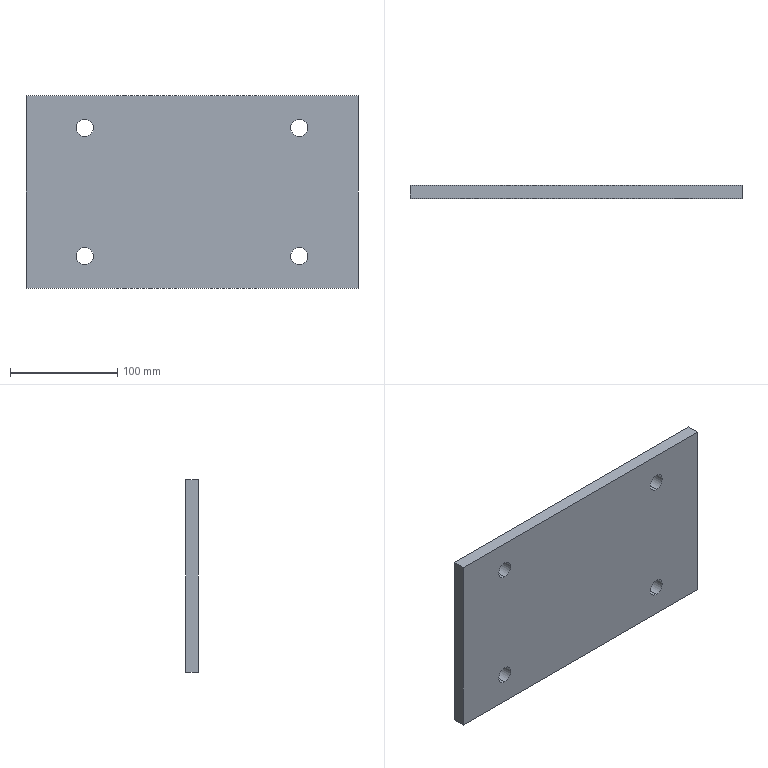Part | SolidWorks | features Extrusion 1 | 1 solid | 14 faces | box 310 x 12 x 180 mm | volume 659949 mm3 | cylinder 8 | plane 6 | commonest cylinder face diameters 16 x8
STEP:
#1=CARTESIAN_POINT('',(100.,6.,-68.));
#2=VERTEX_POINT('',#1);
#3=CARTESIAN_POINT('',(100.,6.,-52.));
#4=VERTEX_POINT('',#3);
#5=CARTESIAN_POINT('',(100.,6.,-60.));
#6=DIRECTION('',(0.,1.,0.));
#7=DIRECTION('',(0.,0.,1.));
#8=AXIS2_PLACEMENT_3D('',#5,#6,#7);
#9=CIRCLE('',#8,8.);
#10=EDGE_CURVE('',#2,#4,#9,.T.);
#11=ORIENTED_EDGE('',*,*,#10,.T.);
#12=CARTESIAN_POINT('',(100.,-6.,-52.));
#13=VERTEX_POINT('',#12);
#14=CARTESIAN_POINT('',(100.,6.,-52.));
#15=DIRECTION('',(0.,-1.,0.));
#16=VECTOR('',#15,1000.);
#17=LINE('',#14,#16);
#18=EDGE_CURVE('',#4,#13,#17,.T.);
#19=ORIENTED_EDGE('',*,*,#18,.T.);
#20=CARTESIAN_POINT('',(100.,-6.,-68.));
#21=VERTEX_POINT('',#20);
#22=CARTESIAN_POINT('',(100.,-6.,-60.));
#23=DIRECTION('',(0.,1.,0.));
#24=DIRECTION('',(0.,0.,1.));
#25=AXIS2_PLACEMENT_3D('',#22,#23,#24);
#26=CIRCLE('',#25,8.);
#27=EDGE_CURVE('',#21,#13,#26,.T.);
#28=ORIENTED_EDGE('',*,*,#27,.F.);
#29=CARTESIAN_POINT('',(100.,6.,-68.));
#30=DIRECTION('',(0.,-1.,0.));
#31=VECTOR('',#30,1000.);
#32=LINE('',#29,#31);
#33=EDGE_CURVE('',#2,#21,#32,.T.);
#34=ORIENTED_EDGE('',*,*,#33,.F.);
#35=EDGE_LOOP('',(#11,#19,#28,#34));
#36=FACE_OUTER_BOUND('',#35,.T.);
#37=CARTESIAN_POINT('',(100.,6.,-60.));
#38=DIRECTION('',(0.,-1.,0.));
#39=DIRECTION('',(0.,0.,-1.));
#40=AXIS2_PLACEMENT_3D('',#37,#38,#39);
#41=CYLINDRICAL_SURFACE('',#40,8.);
#42=ADVANCED_FACE('',(#36),#41,.F.);
#43=CARTESIAN_POINT('',(-100.,6.,-68.));
#44=VERTEX_POINT('',#43);
#45=CARTESIAN_POINT('',(-100.,6.,-52.));
#46=VERTEX_POINT('',#45);
#47=CARTESIAN_POINT('',(-100.,6.,-60.));
#48=DIRECTION('',(0.,1.,0.));
#49=DIRECTION('',(0.,0.,1.));
#50=AXIS2_PLACEMENT_3D('',#47,#48,#49);
#51=CIRCLE('',#50,8.);
#52=EDGE_CURVE('',#44,#46,#51,.T.);
#53=ORIENTED_EDGE('',*,*,#52,.T.);
#54=CARTESIAN_POINT('',(-100.,-6.,-52.));
#55=VERTEX_POINT('',#54);
#56=CARTESIAN_POINT('',(-100.,6.,-52.));
#57=DIRECTION('',(0.,-1.,0.));
#58=VECTOR('',#57,1000.);
#59=LINE('',#56,#58);
#60=EDGE_CURVE('',#46,#55,#59,.T.);
#61=ORIENTED_EDGE('',*,*,#60,.T.);
#62=CARTESIAN_POINT('',(-100.,-6.,-68.));
#63=VERTEX_POINT('',#62);
#64=CARTESIAN_POINT('',(-100.,-6.,-60.));
#65=DIRECTION('',(0.,1.,0.));
#66=DIRECTION('',(0.,0.,1.));
#67=AXIS2_PLACEMENT_3D('',#64,#65,#66);
#68=CIRCLE('',#67,8.);
#69=EDGE_CURVE('',#63,#55,#68,.T.);
#70=ORIENTED_EDGE('',*,*,#69,.F.);
#71=CARTESIAN_POINT('',(-100.,6.,-68.));
#72=DIRECTION('',(0.,-1.,0.));
#73=VECTOR('',#72,1000.);
#74=LINE('',#71,#73);
#75=EDGE_CURVE('',#44,#63,#74,.T.);
#76=ORIENTED_EDGE('',*,*,#75,.F.);
#77=EDGE_LOOP('',(#53,#61,#70,#76));
#78=FACE_OUTER_BOUND('',#77,.T.);
#79=CARTESIAN_POINT('',(-100.,6.,-60.));
#80=DIRECTION('',(0.,-1.,0.));
#81=DIRECTION('',(0.,0.,-1.));
#82=AXIS2_PLACEMENT_3D('',#79,#80,#81);
#83=CYLINDRICAL_SURFACE('',#82,8.);
#84=ADVANCED_FACE('',(#78),#83,.F.);
#85=CARTESIAN_POINT('',(-100.,6.,52.));
#86=VERTEX_POINT('',#85);
#87=CARTESIAN_POINT('',(-100.,6.,68.));
#88=VERTEX_POINT('',#87);
#89=CARTESIAN_POINT('',(-100.,6.,60.));
#90=DIRECTION('',(0.,1.,0.));
#91=DIRECTION('',(0.,0.,1.));
#92=AXIS2_PLACEMENT_3D('',#89,#90,#91);
#93=CIRCLE('',#92,8.);
#94=EDGE_CURVE('',#86,#88,#93,.T.);
#95=ORIENTED_EDGE('',*,*,#94,.T.);
#96=CARTESIAN_POINT('',(-100.,-6.,68.));
#97=VERTEX_POINT('',#96);
#98=CARTESIAN_POINT('',(-100.,6.,68.));
#99=DIRECTION('',(0.,-1.,0.));
#100=VECTOR('',#99,1000.);
#101=LINE('',#98,#100);
#102=EDGE_CURVE('',#88,#97,#101,.T.);
#103=ORIENTED_EDGE('',*,*,#102,.T.);
#104=CARTESIAN_POINT('',(-100.,-6.,52.));
#105=VERTEX_POINT('',#104);
#106=CARTESIAN_POINT('',(-100.,-6.,60.));
#107=DIRECTION('',(0.,1.,0.));
#108=DIRECTION('',(0.,0.,1.));
#109=AXIS2_PLACEMENT_3D('',#106,#107,#108);
#110=CIRCLE('',#109,8.);
#111=EDGE_CURVE('',#105,#97,#110,.T.);
#112=ORIENTED_EDGE('',*,*,#111,.F.);
#113=CARTESIAN_POINT('',(-100.,6.,52.));
#114=DIRECTION('',(0.,-1.,0.));
#115=VECTOR('',#114,1000.);
#116=LINE('',#113,#115);
#117=EDGE_CURVE('',#86,#105,#116,.T.);
#118=ORIENTED_EDGE('',*,*,#117,.F.);
#119=EDGE_LOOP('',(#95,#103,#112,#118));
#120=FACE_OUTER_BOUND('',#119,.T.);
#121=CARTESIAN_POINT('',(-100.,6.,60.));
#122=DIRECTION('',(0.,-1.,0.));
#123=DIRECTION('',(0.,0.,-1.));
#124=AXIS2_PLACEMENT_3D('',#121,#122,#123);
#125=CYLINDRICAL_SURFACE('',#124,8.);
#126=ADVANCED_FACE('',(#120),#125,.F.);
#127=CARTESIAN_POINT('',(100.,6.,52.));
#128=VERTEX_POINT('',#127);
#129=CARTESIAN_POINT('',(100.,6.,68.));
#130=VERTEX_POINT('',#129);
#131=CARTESIAN_POINT('',(100.,6.,60.));
#132=DIRECTION('',(0.,1.,0.));
#133=DIRECTION('',(0.,0.,1.));
#134=AXIS2_PLACEMENT_3D('',#131,#132,#133);
#135=CIRCLE('',#134,8.);
#136=EDGE_CURVE('',#128,#130,#135,.T.);
#137=ORIENTED_EDGE('',*,*,#136,.T.);
#138=CARTESIAN_POINT('',(100.,-6.,68.));
#139=VERTEX_POINT('',#138);
#140=CARTESIAN_POINT('',(100.,6.,68.));
#141=DIRECTION('',(0.,-1.,0.));
#142=VECTOR('',#141,1000.);
#143=LINE('',#140,#142);
#144=EDGE_CURVE('',#130,#139,#143,.T.);
#145=ORIENTED_EDGE('',*,*,#144,.T.);
#146=CARTESIAN_POINT('',(100.,-6.,52.));
#147=VERTEX_POINT('',#146);
#148=CARTESIAN_POINT('',(100.,-6.,60.));
#149=DIRECTION('',(0.,1.,0.));
#150=DIRECTION('',(0.,0.,1.));
#151=AXIS2_PLACEMENT_3D('',#148,#149,#150);
#152=CIRCLE('',#151,8.);
#153=EDGE_CURVE('',#147,#139,#152,.T.);
#154=ORIENTED_EDGE('',*,*,#153,.F.);
#155=CARTESIAN_POINT('',(100.,6.,52.));
#156=DIRECTION('',(0.,-1.,0.));
#157=VECTOR('',#156,1000.);
#158=LINE('',#155,#157);
#159=EDGE_CURVE('',#128,#147,#158,.T.);
#160=ORIENTED_EDGE('',*,*,#159,.F.);
#161=EDGE_LOOP('',(#137,#145,#154,#160));
#162=FACE_OUTER_BOUND('',#161,.T.);
#163=CARTESIAN_POINT('',(100.,6.,60.));
#164=DIRECTION('',(0.,-1.,0.));
#165=DIRECTION('',(0.,0.,-1.));
#166=AXIS2_PLACEMENT_3D('',#163,#164,#165);
#167=CYLINDRICAL_SURFACE('',#166,8.);
#168=ADVANCED_FACE('',(#162),#167,.F.);
#169=ORIENTED_EDGE('',*,*,#52,.F.);
#170=CARTESIAN_POINT('',(-100.,6.,-60.));
#171=DIRECTION('',(0.,1.,0.));
#172=DIRECTION('',(0.,0.,1.));
#173=AXIS2_PLACEMENT_3D('',#170,#171,#172);
#174=CIRCLE('',#173,8.);
#175=EDGE_CURVE('',#46,#44,#174,.T.);
#176=ORIENTED_EDGE('',*,*,#175,.F.);
#177=EDGE_LOOP('',(#169,#176));
#178=FACE_BOUND('',#177,.T.);
#179=ORIENTED_EDGE('',*,*,#136,.F.);
#180=CARTESIAN_POINT('',(100.,6.,60.));
#181=DIRECTION('',(0.,1.,0.));
#182=DIRECTION('',(0.,0.,1.));
#183=AXIS2_PLACEMENT_3D('',#180,#181,#182);
#184=CIRCLE('',#183,8.);
#185=EDGE_CURVE('',#130,#128,#184,.T.);
#186=ORIENTED_EDGE('',*,*,#185,.F.);
#187=EDGE_LOOP('',(#179,#186));
#188=FACE_BOUND('',#187,.T.);
#189=CARTESIAN_POINT('',(-155.,6.,-90.));
#190=VERTEX_POINT('',#189);
#191=CARTESIAN_POINT('',(-155.,6.,90.));
#192=VERTEX_POINT('',#191);
#193=CARTESIAN_POINT('',(-155.,6.,90.));
#194=DIRECTION('',(0.,0.,1.));
#195=VECTOR('',#194,1000.);
#196=LINE('',#193,#195);
#197=EDGE_CURVE('',#190,#192,#196,.T.);
#198=ORIENTED_EDGE('',*,*,#197,.T.);
#199=CARTESIAN_POINT('',(155.,6.,90.));
#200=VERTEX_POINT('',#199);
#201=CARTESIAN_POINT('',(155.,6.,90.));
#202=DIRECTION('',(1.,0.,0.));
#203=VECTOR('',#202,1000.);
#204=LINE('',#201,#203);
#205=EDGE_CURVE('',#192,#200,#204,.T.);
#206=ORIENTED_EDGE('',*,*,#205,.T.);
#207=CARTESIAN_POINT('',(155.,6.,-90.));
#208=VERTEX_POINT('',#207);
#209=CARTESIAN_POINT('',(155.,6.,-90.));
#210=DIRECTION('',(0.,0.,-1.));
#211=VECTOR('',#210,1000.);
#212=LINE('',#209,#211);
#213=EDGE_CURVE('',#200,#208,#212,.T.);
#214=ORIENTED_EDGE('',*,*,#213,.T.);
#215=CARTESIAN_POINT('',(-155.,6.,-90.));
#216=DIRECTION('',(-1.,0.,0.));
#217=VECTOR('',#216,1000.);
#218=LINE('',#215,#217);
#219=EDGE_CURVE('',#208,#190,#218,.T.);
#220=ORIENTED_EDGE('',*,*,#219,.T.);
#221=EDGE_LOOP('',(#198,#206,#214,#220));
#222=FACE_OUTER_BOUND('',#221,.T.);
#223=ORIENTED_EDGE('',*,*,#94,.F.);
#224=CARTESIAN_POINT('',(-100.,6.,60.));
#225=DIRECTION('',(0.,1.,0.));
#226=DIRECTION('',(0.,0.,1.));
#227=AXIS2_PLACEMENT_3D('',#224,#225,#226);
#228=CIRCLE('',#227,8.);
#229=EDGE_CURVE('',#88,#86,#228,.T.);
#230=ORIENTED_EDGE('',*,*,#229,.F.);
#231=EDGE_LOOP('',(#223,#230));
#232=FACE_BOUND('',#231,.T.);
#233=ORIENTED_EDGE('',*,*,#10,.F.);
#234=CARTESIAN_POINT('',(100.,6.,-60.));
#235=DIRECTION('',(0.,1.,0.));
#236=DIRECTION('',(0.,0.,1.));
#237=AXIS2_PLACEMENT_3D('',#234,#235,#236);
#238=CIRCLE('',#237,8.);
#239=EDGE_CURVE('',#4,#2,#238,.T.);
#240=ORIENTED_EDGE('',*,*,#239,.F.);
#241=EDGE_LOOP('',(#233,#240));
#242=FACE_BOUND('',#241,.T.);
#243=CARTESIAN_POINT('',(-155.,6.,-90.));
#244=DIRECTION('',(0.,-1.,0.));
#245=DIRECTION('',(0.,0.,-1.));
#246=AXIS2_PLACEMENT_3D('',#243,#244,#245);
#247=PLANE('',#246);
#248=ADVANCED_FACE('',(#178,#188,#222,#232,#242),#247,.F.);
#249=ORIENTED_EDGE('',*,*,#69,.T.);
#250=CARTESIAN_POINT('',(-100.,-6.,-60.));
#251=DIRECTION('',(0.,1.,0.));
#252=DIRECTION('',(0.,0.,1.));
#253=AXIS2_PLACEMENT_3D('',#250,#251,#252);
#254=CIRCLE('',#253,8.);
#255=EDGE_CURVE('',#55,#63,#254,.T.);
#256=ORIENTED_EDGE('',*,*,#255,.T.);
#257=EDGE_LOOP('',(#249,#256));
#258=FACE_BOUND('',#257,.T.);
#259=ORIENTED_EDGE('',*,*,#153,.T.);
#260=CARTESIAN_POINT('',(100.,-6.,60.));
#261=DIRECTION('',(0.,1.,0.));
#262=DIRECTION('',(0.,0.,1.));
#263=AXIS2_PLACEMENT_3D('',#260,#261,#262);
#264=CIRCLE('',#263,8.);
#265=EDGE_CURVE('',#139,#147,#264,.T.);
#266=ORIENTED_EDGE('',*,*,#265,.T.);
#267=EDGE_LOOP('',(#259,#266));
#268=FACE_BOUND('',#267,.T.);
#269=CARTESIAN_POINT('',(-155.,-6.,-90.));
#270=VERTEX_POINT('',#269);
#271=CARTESIAN_POINT('',(-155.,-6.,90.));
#272=VERTEX_POINT('',#271);
#273=CARTESIAN_POINT('',(-155.,-6.,90.));
#274=DIRECTION('',(0.,0.,1.));
#275=VECTOR('',#274,1000.);
#276=LINE('',#273,#275);
#277=EDGE_CURVE('',#270,#272,#276,.T.);
#278=ORIENTED_EDGE('',*,*,#277,.F.);
#279=CARTESIAN_POINT('',(155.,-6.,-90.));
#280=VERTEX_POINT('',#279);
#281=CARTESIAN_POINT('',(-155.,-6.,-90.));
#282=DIRECTION('',(-1.,0.,0.));
#283=VECTOR('',#282,1000.);
#284=LINE('',#281,#283);
#285=EDGE_CURVE('',#280,#270,#284,.T.);
#286=ORIENTED_EDGE('',*,*,#285,.F.);
#287=CARTESIAN_POINT('',(155.,-6.,90.));
#288=VERTEX_POINT('',#287);
#289=CARTESIAN_POINT('',(155.,-6.,-90.));
#290=DIRECTION('',(0.,0.,-1.));
#291=VECTOR('',#290,1000.);
#292=LINE('',#289,#291);
#293=EDGE_CURVE('',#288,#280,#292,.T.);
#294=ORIENTED_EDGE('',*,*,#293,.F.);
#295=CARTESIAN_POINT('',(155.,-6.,90.));
#296=DIRECTION('',(1.,0.,0.));
#297=VECTOR('',#296,1000.);
#298=LINE('',#295,#297);
#299=EDGE_CURVE('',#272,#288,#298,.T.);
#300=ORIENTED_EDGE('',*,*,#299,.F.);
#301=EDGE_LOOP('',(#278,#286,#294,#300));
#302=FACE_OUTER_BOUND('',#301,.T.);
#303=ORIENTED_EDGE('',*,*,#111,.T.);
#304=CARTESIAN_POINT('',(-100.,-6.,60.));
#305=DIRECTION('',(0.,1.,0.));
#306=DIRECTION('',(0.,0.,1.));
#307=AXIS2_PLACEMENT_3D('',#304,#305,#306);
#308=CIRCLE('',#307,8.);
#309=EDGE_CURVE('',#97,#105,#308,.T.);
#310=ORIENTED_EDGE('',*,*,#309,.T.);
#311=EDGE_LOOP('',(#303,#310));
#312=FACE_BOUND('',#311,.T.);
#313=ORIENTED_EDGE('',*,*,#27,.T.);
#314=CARTESIAN_POINT('',(100.,-6.,-60.));
#315=DIRECTION('',(0.,1.,0.));
#316=DIRECTION('',(0.,0.,1.));
#317=AXIS2_PLACEMENT_3D('',#314,#315,#316);
#318=CIRCLE('',#317,8.);
#319=EDGE_CURVE('',#13,#21,#318,.T.);
#320=ORIENTED_EDGE('',*,*,#319,.T.);
#321=EDGE_LOOP('',(#313,#320));
#322=FACE_BOUND('',#321,.T.);
#323=CARTESIAN_POINT('',(-155.,-6.,-90.));
#324=DIRECTION('',(0.,-1.,0.));
#325=DIRECTION('',(0.,0.,-1.));
#326=AXIS2_PLACEMENT_3D('',#323,#324,#325);
#327=PLANE('',#326);
#328=ADVANCED_FACE('',(#258,#268,#302,#312,#322),#327,.T.);
#329=ORIENTED_EDGE('',*,*,#277,.T.);
#330=CARTESIAN_POINT('',(-155.,6.,90.));
#331=DIRECTION('',(0.,-1.,0.));
#332=VECTOR('',#331,1000.);
#333=LINE('',#330,#332);
#334=EDGE_CURVE('',#192,#272,#333,.T.);
#335=ORIENTED_EDGE('',*,*,#334,.F.);
#336=ORIENTED_EDGE('',*,*,#197,.F.);
#337=CARTESIAN_POINT('',(-155.,6.,-90.));
#338=DIRECTION('',(0.,-1.,0.));
#339=VECTOR('',#338,1000.);
#340=LINE('',#337,#339);
#341=EDGE_CURVE('',#190,#270,#340,.T.);
#342=ORIENTED_EDGE('',*,*,#341,.T.);
#343=EDGE_LOOP('',(#329,#335,#336,#342));
#344=FACE_OUTER_BOUND('',#343,.T.);
#345=CARTESIAN_POINT('',(-155.,6.,90.));
#346=DIRECTION('',(1.,0.,0.));
#347=DIRECTION('',(0.,0.,-1.));
#348=AXIS2_PLACEMENT_3D('',#345,#346,#347);
#349=PLANE('',#348);
#350=ADVANCED_FACE('',(#344),#349,.F.);
#351=ORIENTED_EDGE('',*,*,#299,.T.);
#352=CARTESIAN_POINT('',(155.,6.,90.));
#353=DIRECTION('',(0.,-1.,0.));
#354=VECTOR('',#353,1000.);
#355=LINE('',#352,#354);
#356=EDGE_CURVE('',#200,#288,#355,.T.);
#357=ORIENTED_EDGE('',*,*,#356,.F.);
#358=ORIENTED_EDGE('',*,*,#205,.F.);
#359=ORIENTED_EDGE('',*,*,#334,.T.);
#360=EDGE_LOOP('',(#351,#357,#358,#359));
#361=FACE_OUTER_BOUND('',#360,.T.);
#362=CARTESIAN_POINT('',(155.,6.,90.));
#363=DIRECTION('',(0.,0.,-1.));
#364=DIRECTION('',(-1.,0.,0.));
#365=AXIS2_PLACEMENT_3D('',#362,#363,#364);
#366=PLANE('',#365);
#367=ADVANCED_FACE('',(#361),#366,.F.);
#368=ORIENTED_EDGE('',*,*,#293,.T.);
#369=CARTESIAN_POINT('',(155.,6.,-90.));
#370=DIRECTION('',(0.,-1.,0.));
#371=VECTOR('',#370,1000.);
#372=LINE('',#369,#371);
#373=EDGE_CURVE('',#208,#280,#372,.T.);
#374=ORIENTED_EDGE('',*,*,#373,.F.);
#375=ORIENTED_EDGE('',*,*,#213,.F.);
#376=ORIENTED_EDGE('',*,*,#356,.T.);
#377=EDGE_LOOP('',(#368,#374,#375,#376));
#378=FACE_OUTER_BOUND('',#377,.T.);
#379=CARTESIAN_POINT('',(155.,6.,-90.));
#380=DIRECTION('',(-1.,0.,0.));
#381=DIRECTION('',(0.,0.,1.));
#382=AXIS2_PLACEMENT_3D('',#379,#380,#381);
#383=PLANE('',#382);
#384=ADVANCED_FACE('',(#378),#383,.F.);
#385=ORIENTED_EDGE('',*,*,#285,.T.);
#386=ORIENTED_EDGE('',*,*,#341,.F.);
#387=ORIENTED_EDGE('',*,*,#219,.F.);
#388=ORIENTED_EDGE('',*,*,#373,.T.);
#389=EDGE_LOOP('',(#385,#386,#387,#388));
#390=FACE_OUTER_BOUND('',#389,.T.);
#391=CARTESIAN_POINT('',(-155.,6.,-90.));
#392=DIRECTION('',(0.,0.,1.));
#393=DIRECTION('',(1.,0.,0.));
#394=AXIS2_PLACEMENT_3D('',#391,#392,#393);
#395=PLANE('',#394);
#396=ADVANCED_FACE('',(#390),#395,.F.);
#397=ORIENTED_EDGE('',*,*,#144,.F.);
#398=ORIENTED_EDGE('',*,*,#185,.T.);
#399=ORIENTED_EDGE('',*,*,#159,.T.);
#400=ORIENTED_EDGE('',*,*,#265,.F.);
#401=EDGE_LOOP('',(#397,#398,#399,#400));
#402=FACE_OUTER_BOUND('',#401,.T.);
#403=CARTESIAN_POINT('',(100.,6.,60.));
#404=DIRECTION('',(0.,-1.,0.));
#405=DIRECTION('',(0.,0.,-1.));
#406=AXIS2_PLACEMENT_3D('',#403,#404,#405);
#407=CYLINDRICAL_SURFACE('',#406,8.);
#408=ADVANCED_FACE('',(#402),#407,.F.);
#409=ORIENTED_EDGE('',*,*,#102,.F.);
#410=ORIENTED_EDGE('',*,*,#229,.T.);
#411=ORIENTED_EDGE('',*,*,#117,.T.);
#412=ORIENTED_EDGE('',*,*,#309,.F.);
#413=EDGE_LOOP('',(#409,#410,#411,#412));
#414=FACE_OUTER_BOUND('',#413,.T.);
#415=CARTESIAN_POINT('',(-100.,6.,60.));
#416=DIRECTION('',(0.,-1.,0.));
#417=DIRECTION('',(0.,0.,-1.));
#418=AXIS2_PLACEMENT_3D('',#415,#416,#417);
#419=CYLINDRICAL_SURFACE('',#418,8.);
#420=ADVANCED_FACE('',(#414),#419,.F.);
#421=ORIENTED_EDGE('',*,*,#60,.F.);
#422=ORIENTED_EDGE('',*,*,#175,.T.);
#423=ORIENTED_EDGE('',*,*,#75,.T.);
#424=ORIENTED_EDGE('',*,*,#255,.F.);
#425=EDGE_LOOP('',(#421,#422,#423,#424));
#426=FACE_OUTER_BOUND('',#425,.T.);
#427=CARTESIAN_POINT('',(-100.,6.,-60.));
#428=DIRECTION('',(0.,-1.,0.));
#429=DIRECTION('',(0.,0.,-1.));
#430=AXIS2_PLACEMENT_3D('',#427,#428,#429);
#431=CYLINDRICAL_SURFACE('',#430,8.);
#432=ADVANCED_FACE('',(#426),#431,.F.);
#433=ORIENTED_EDGE('',*,*,#18,.F.);
#434=ORIENTED_EDGE('',*,*,#239,.T.);
#435=ORIENTED_EDGE('',*,*,#33,.T.);
#436=ORIENTED_EDGE('',*,*,#319,.F.);
#437=EDGE_LOOP('',(#433,#434,#435,#436));
#438=FACE_OUTER_BOUND('',#437,.T.);
#439=CARTESIAN_POINT('',(100.,6.,-60.));
#440=DIRECTION('',(0.,-1.,0.));
#441=DIRECTION('',(0.,0.,-1.));
#442=AXIS2_PLACEMENT_3D('',#439,#440,#441);
#443=CYLINDRICAL_SURFACE('',#442,8.);
#444=ADVANCED_FACE('',(#438),#443,.F.);
#445=CLOSED_SHELL('',(#42,#84,#126,#168,#248,#328,#350,#367,#384,#396,#408,#420,#432,#444));
#446=MANIFOLD_SOLID_BREP('',#445);
#447=CARTESIAN_POINT('',(0.,0.,0.));
#448=DIRECTION('',(0.,0.,1.));
#449=DIRECTION('',(1.,0.,0.));
#450=AXIS2_PLACEMENT_3D('',#447,#448,#449);
#451=(LENGTH_UNIT()NAMED_UNIT(*)SI_UNIT(.MILLI.,.METRE.));
#452=UNCERTAINTY_MEASURE_WITH_UNIT(LENGTH_MEASURE(0.00001),#451,'','');
#453=(NAMED_UNIT(*)PLANE_ANGLE_UNIT()SI_UNIT($,.RADIAN.));
#454=(NAMED_UNIT(*)SI_UNIT($,.STERADIAN.)SOLID_ANGLE_UNIT());
#455=(GEOMETRIC_REPRESENTATION_CONTEXT(3)GLOBAL_UNCERTAINTY_ASSIGNED_CONTEXT((#452))GLOBAL_UNIT_ASSIGNED_CONTEXT((#451,#453,#454))REPRESENTATION_CONTEXT('',''));
#456=ADVANCED_BREP_SHAPE_REPRESENTATION('',(#446,#450),#455);